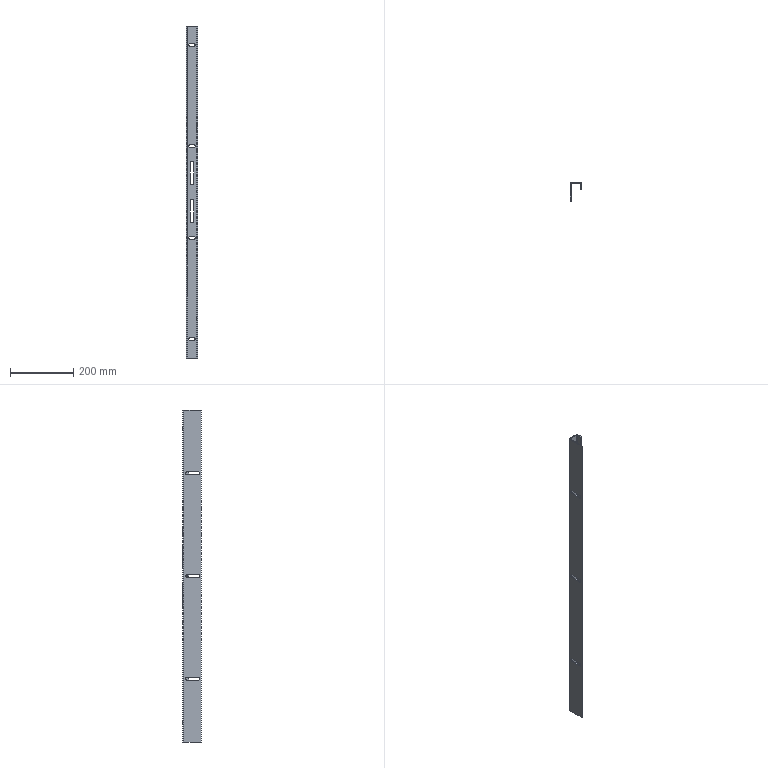Part | SolidWorks | features Cut 2, ICE 2, FlatPattern 1, SMBaseFlange 1, SheetMetal 1 | 1 solid | 72 faces | box 37 x 60 x 1050 mm | volume 331468 mm3 | cylinder 36 | plane 36 | commonest cylinder face diameters 10 x18 6 x10 12 x4 2 x2 8 x2